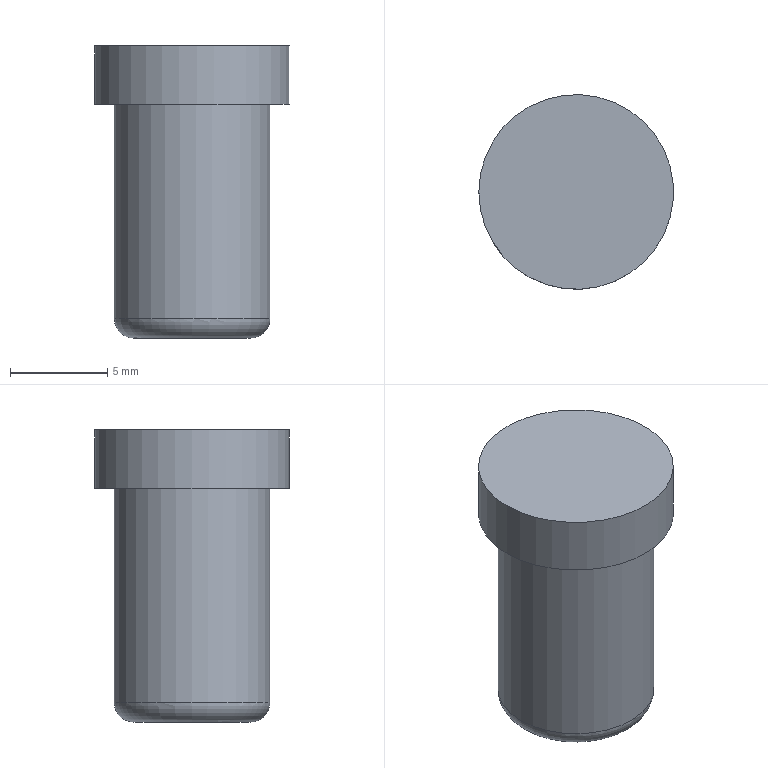Part | STEP file | gslz 2016.10.28-10_id1782_x_t | 1 solid | 6 faces | box 10 x 10 x 15 mm | volume 833.713 mm3 | plane 3 | cylinder 2 | torus 1 | commonest cylinder face diameters 8 x1 10 x1
STEP:
#1=CARTESIAN_POINT('',(0.,0.,0.));
#2=DIRECTION('',(0.,0.,1.));
#3=DIRECTION('',(1.,0.,0.));
#4=AXIS2_PLACEMENT_3D('',#1,#2,#3);
#5=CARTESIAN_POINT('',(815.5,119.5,-4.));
#6=VERTEX_POINT('',#5);
#7=CARTESIAN_POINT('',(819.5,119.5,-4.));
#8=DIRECTION('',(0.,0.,1.));
#9=DIRECTION('',(-1.,0.,0.));
#10=AXIS2_PLACEMENT_3D('',#7,#8,#9);
#11=CIRCLE('',#10,4.);
#12=CARTESIAN_POINT('',(819.5,119.5,-12.));
#13=DIRECTION('',(0.,0.,1.));
#14=DIRECTION('',(1.,0.,0.));
#15=AXIS2_PLACEMENT_3D('',#12,#13,#14);
#16=CYLINDRICAL_SURFACE('',#15,4.);
#17=CARTESIAN_POINT('',(3.142,8.));
#18=DIRECTION('',(1.,0.));
#19=VECTOR('',#18,1.);
#20=LINE('',#17,#19);
#21=(GEOMETRIC_REPRESENTATION_CONTEXT(2)PARAMETRIC_REPRESENTATION_CONTEXT()REPRESENTATION_CONTEXT('',''));
#22=DEFINITIONAL_REPRESENTATION('',(#20),#21);
#23=PCURVE('',#16,#22);
#24=CARTESIAN_POINT('',(819.5,119.5,-4.));
#25=DIRECTION('',(0.,0.,1.));
#26=DIRECTION('',(-1.,0.,0.));
#27=AXIS2_PLACEMENT_3D('',#24,#25,#26);
#28=TOROIDAL_SURFACE('',#27,3.,1.);
#29=CARTESIAN_POINT('',(0.,6.283));
#30=DIRECTION('',(1.,0.));
#31=VECTOR('',#30,1.);
#32=LINE('',#29,#31);
#33=(GEOMETRIC_REPRESENTATION_CONTEXT(2)PARAMETRIC_REPRESENTATION_CONTEXT()REPRESENTATION_CONTEXT('',''));
#34=DEFINITIONAL_REPRESENTATION('',(#32),#33);
#35=PCURVE('',#28,#34);
#36=SURFACE_CURVE('',#11,(#23,#35),.PCURVE_S1.);
#37=EDGE_CURVE('',#6,#6,#36,.T.);
#38=ORIENTED_EDGE('',*,*,#37,.T.);
#39=CARTESIAN_POINT('',(815.5,119.5,7.));
#40=VERTEX_POINT('',#39);
#41=CARTESIAN_POINT('',(815.5,119.5,-4.));
#42=CARTESIAN_POINT('',(815.5,119.5,7.));
#43=B_SPLINE_CURVE_WITH_KNOTS('',1,(#41,#42),.UNSPECIFIED.,.F.,.F.,(2,2),(8.,19.),.PIECEWISE_BEZIER_KNOTS.);
#44=CARTESIAN_POINT('',(9.425,0.));
#45=DIRECTION('',(0.,1.));
#46=VECTOR('',#45,1.);
#47=LINE('',#44,#46);
#48=(GEOMETRIC_REPRESENTATION_CONTEXT(2)PARAMETRIC_REPRESENTATION_CONTEXT()REPRESENTATION_CONTEXT('',''));
#49=DEFINITIONAL_REPRESENTATION('',(#47),#48);
#50=PCURVE('',#16,#49);
#51=CARTESIAN_POINT('',(3.142,0.));
#52=DIRECTION('',(0.,1.));
#53=VECTOR('',#52,1.);
#54=LINE('',#51,#53);
#55=(GEOMETRIC_REPRESENTATION_CONTEXT(2)PARAMETRIC_REPRESENTATION_CONTEXT()REPRESENTATION_CONTEXT('',''));
#56=DEFINITIONAL_REPRESENTATION('',(#54),#55);
#57=PCURVE('',#16,#56);
#58=SEAM_CURVE('',#43,(#50,#57),.PCURVE_S1.);
#59=EDGE_CURVE('',#6,#40,#58,.T.);
#60=ORIENTED_EDGE('',*,*,#59,.T.);
#61=CARTESIAN_POINT('',(819.5,119.5,7.));
#62=DIRECTION('',(0.,0.,1.));
#63=DIRECTION('',(-1.,0.,0.));
#64=AXIS2_PLACEMENT_3D('',#61,#62,#63);
#65=CIRCLE('',#64,4.);
#66=CARTESIAN_POINT('',(3.142,19.));
#67=DIRECTION('',(1.,0.));
#68=VECTOR('',#67,1.);
#69=LINE('',#66,#68);
#70=(GEOMETRIC_REPRESENTATION_CONTEXT(2)PARAMETRIC_REPRESENTATION_CONTEXT()REPRESENTATION_CONTEXT('',''));
#71=DEFINITIONAL_REPRESENTATION('',(#69),#70);
#72=PCURVE('',#16,#71);
#73=CARTESIAN_POINT('',(819.5,119.5,7.));
#74=DIRECTION('',(0.,0.,1.));
#75=DIRECTION('',(1.,0.,0.));
#76=AXIS2_PLACEMENT_3D('',#73,#74,#75);
#77=PLANE('',#76);
#78=CARTESIAN_POINT('',(0.,0.));
#79=DIRECTION('',(-1.,0.));
#80=AXIS2_PLACEMENT_2D('',#78,#79);
#81=CIRCLE('',#80,4.);
#82=(GEOMETRIC_REPRESENTATION_CONTEXT(2)PARAMETRIC_REPRESENTATION_CONTEXT()REPRESENTATION_CONTEXT('',''));
#83=DEFINITIONAL_REPRESENTATION('',(#81),#82);
#84=PCURVE('',#77,#83);
#85=SURFACE_CURVE('',#65,(#72,#84),.PCURVE_S1.);
#86=EDGE_CURVE('',#40,#40,#85,.T.);
#87=ORIENTED_EDGE('',*,*,#86,.F.);
#88=ORIENTED_EDGE('',*,*,#59,.F.);
#89=EDGE_LOOP('',(#38,#60,#87,#88));
#90=FACE_BOUND('',#89,.T.);
#91=ADVANCED_FACE('',(#90),#16,.T.);
#92=CARTESIAN_POINT('',(822.5,119.5,-5.));
#93=VERTEX_POINT('',#92);
#94=CARTESIAN_POINT('',(816.5,119.5,-5.));
#95=VERTEX_POINT('',#94);
#96=CARTESIAN_POINT('',(819.5,119.5,-5.));
#97=DIRECTION('',(0.,0.,-1.));
#98=DIRECTION('',(-1.,0.,0.));
#99=AXIS2_PLACEMENT_3D('',#96,#97,#98);
#100=CIRCLE('',#99,3.);
#101=CARTESIAN_POINT('',(819.5,119.5,-5.));
#102=DIRECTION('',(0.,0.,1.));
#103=DIRECTION('',(1.,0.,0.));
#104=AXIS2_PLACEMENT_3D('',#101,#102,#103);
#105=PLANE('',#104);
#106=CARTESIAN_POINT('',(-3.,0.));
#107=CARTESIAN_POINT('',(-3.,5.196));
#108=CARTESIAN_POINT('',(1.5,2.598));
#109=CARTESIAN_POINT('',(6.,0.));
#110=CARTESIAN_POINT('',(1.5,-2.598));
#111=CARTESIAN_POINT('',(-3.,-5.196));
#112=CARTESIAN_POINT('',(-3.,0.));
#113=(BOUNDED_CURVE()B_SPLINE_CURVE(2,(#106,#107,#108,#109,#110,#111,#112),.UNSPECIFIED.,.T.,.F.)B_SPLINE_CURVE_WITH_KNOTS((1,2,2,2,2,1),(-2.094,0.,2.094,4.189,6.283,8.378),.UNSPECIFIED.)CURVE()GEOMETRIC_REPRESENTATION_ITEM()RATIONAL_B_SPLINE_CURVE((1.,0.5,1.,0.5,1.,0.5,1.))REPRESENTATION_ITEM(''));
#114=(GEOMETRIC_REPRESENTATION_CONTEXT(2)PARAMETRIC_REPRESENTATION_CONTEXT()REPRESENTATION_CONTEXT('',''));
#115=DEFINITIONAL_REPRESENTATION('',(#113),#114);
#116=PCURVE('',#105,#115);
#117=CARTESIAN_POINT('',(6.283,4.712));
#118=DIRECTION('',(-1.,0.));
#119=VECTOR('',#118,1.);
#120=LINE('',#117,#119);
#121=(GEOMETRIC_REPRESENTATION_CONTEXT(2)PARAMETRIC_REPRESENTATION_CONTEXT()REPRESENTATION_CONTEXT('',''));
#122=DEFINITIONAL_REPRESENTATION('',(#120),#121);
#123=PCURVE('',#28,#122);
#124=SURFACE_CURVE('',#100,(#116,#123),.PCURVE_S1.);
#125=EDGE_CURVE('',#93,#95,#124,.T.);
#126=ORIENTED_EDGE('',*,*,#125,.T.);
#127=CARTESIAN_POINT('',(819.5,119.5,-5.));
#128=DIRECTION('',(0.,0.,-1.));
#129=DIRECTION('',(-1.,0.,0.));
#130=AXIS2_PLACEMENT_3D('',#127,#128,#129);
#131=CIRCLE('',#130,3.);
#132=CARTESIAN_POINT('',(-3.,0.));
#133=CARTESIAN_POINT('',(-3.,5.196));
#134=CARTESIAN_POINT('',(1.5,2.598));
#135=CARTESIAN_POINT('',(6.,0.));
#136=CARTESIAN_POINT('',(1.5,-2.598));
#137=CARTESIAN_POINT('',(-3.,-5.196));
#138=CARTESIAN_POINT('',(-3.,0.));
#139=(BOUNDED_CURVE()B_SPLINE_CURVE(2,(#132,#133,#134,#135,#136,#137,#138),.UNSPECIFIED.,.T.,.F.)B_SPLINE_CURVE_WITH_KNOTS((1,2,2,2,2,1),(-2.094,0.,2.094,4.189,6.283,8.378),.UNSPECIFIED.)CURVE()GEOMETRIC_REPRESENTATION_ITEM()RATIONAL_B_SPLINE_CURVE((1.,0.5,1.,0.5,1.,0.5,1.))REPRESENTATION_ITEM(''));
#140=(GEOMETRIC_REPRESENTATION_CONTEXT(2)PARAMETRIC_REPRESENTATION_CONTEXT()REPRESENTATION_CONTEXT('',''));
#141=DEFINITIONAL_REPRESENTATION('',(#139),#140);
#142=PCURVE('',#105,#141);
#143=CARTESIAN_POINT('',(12.566,4.712));
#144=DIRECTION('',(-1.,0.));
#145=VECTOR('',#144,1.);
#146=LINE('',#143,#145);
#147=(GEOMETRIC_REPRESENTATION_CONTEXT(2)PARAMETRIC_REPRESENTATION_CONTEXT()REPRESENTATION_CONTEXT('',''));
#148=DEFINITIONAL_REPRESENTATION('',(#146),#147);
#149=PCURVE('',#28,#148);
#150=SURFACE_CURVE('',#131,(#142,#149),.PCURVE_S1.);
#151=EDGE_CURVE('',#95,#93,#150,.T.);
#152=ORIENTED_EDGE('',*,*,#151,.T.);
#153=EDGE_LOOP('',(#126,#152));
#154=FACE_BOUND('',#153,.T.);
#155=ADVANCED_FACE('',(#154),#105,.F.);
#156=CARTESIAN_POINT('',(814.5,119.5,7.));
#157=VERTEX_POINT('',#156);
#158=CARTESIAN_POINT('',(819.5,119.5,7.));
#159=DIRECTION('',(0.,0.,1.));
#160=DIRECTION('',(-1.,0.,0.));
#161=AXIS2_PLACEMENT_3D('',#158,#159,#160);
#162=CIRCLE('',#161,5.);
#163=CARTESIAN_POINT('',(0.,0.));
#164=DIRECTION('',(-1.,0.));
#165=AXIS2_PLACEMENT_2D('',#163,#164);
#166=CIRCLE('',#165,5.);
#167=(GEOMETRIC_REPRESENTATION_CONTEXT(2)PARAMETRIC_REPRESENTATION_CONTEXT()REPRESENTATION_CONTEXT('',''));
#168=DEFINITIONAL_REPRESENTATION('',(#166),#167);
#169=PCURVE('',#77,#168);
#170=CARTESIAN_POINT('',(819.5,119.5,10.));
#171=DIRECTION('',(0.,0.,-1.));
#172=DIRECTION('',(-1.,0.,0.));
#173=AXIS2_PLACEMENT_3D('',#170,#171,#172);
#174=CYLINDRICAL_SURFACE('',#173,5.);
#175=CARTESIAN_POINT('',(6.283,3.));
#176=DIRECTION('',(-1.,0.));
#177=VECTOR('',#176,1.);
#178=LINE('',#175,#177);
#179=(GEOMETRIC_REPRESENTATION_CONTEXT(2)PARAMETRIC_REPRESENTATION_CONTEXT()REPRESENTATION_CONTEXT('',''));
#180=DEFINITIONAL_REPRESENTATION('',(#178),#179);
#181=PCURVE('',#174,#180);
#182=SURFACE_CURVE('',#162,(#169,#181),.PCURVE_S1.);
#183=EDGE_CURVE('',#157,#157,#182,.T.);
#184=ORIENTED_EDGE('',*,*,#183,.F.);
#185=EDGE_LOOP('',(#184));
#186=FACE_BOUND('',#185,.T.);
#187=ORIENTED_EDGE('',*,*,#86,.T.);
#188=EDGE_LOOP('',(#187));
#189=FACE_BOUND('',#188,.T.);
#190=ADVANCED_FACE('',(#186,#189),#77,.F.);
#191=CARTESIAN_POINT('',(814.5,119.5,10.));
#192=VERTEX_POINT('',#191);
#193=CARTESIAN_POINT('',(819.5,119.5,10.));
#194=DIRECTION('',(0.,0.,1.));
#195=DIRECTION('',(-1.,0.,0.));
#196=AXIS2_PLACEMENT_3D('',#193,#194,#195);
#197=CIRCLE('',#196,5.);
#198=CARTESIAN_POINT('',(6.283,0.));
#199=DIRECTION('',(-1.,0.));
#200=VECTOR('',#199,1.);
#201=LINE('',#198,#200);
#202=(GEOMETRIC_REPRESENTATION_CONTEXT(2)PARAMETRIC_REPRESENTATION_CONTEXT()REPRESENTATION_CONTEXT('',''));
#203=DEFINITIONAL_REPRESENTATION('',(#201),#202);
#204=PCURVE('',#174,#203);
#205=CARTESIAN_POINT('',(819.5,119.5,10.));
#206=DIRECTION('',(0.,0.,1.));
#207=DIRECTION('',(1.,0.,0.));
#208=AXIS2_PLACEMENT_3D('',#205,#206,#207);
#209=PLANE('',#208);
#210=CARTESIAN_POINT('',(0.,0.));
#211=DIRECTION('',(-1.,0.));
#212=AXIS2_PLACEMENT_2D('',#210,#211);
#213=CIRCLE('',#212,5.);
#214=(GEOMETRIC_REPRESENTATION_CONTEXT(2)PARAMETRIC_REPRESENTATION_CONTEXT()REPRESENTATION_CONTEXT('',''));
#215=DEFINITIONAL_REPRESENTATION('',(#213),#214);
#216=PCURVE('',#209,#215);
#217=SURFACE_CURVE('',#197,(#204,#216),.PCURVE_S1.);
#218=EDGE_CURVE('',#192,#192,#217,.T.);
#219=ORIENTED_EDGE('',*,*,#218,.F.);
#220=CARTESIAN_POINT('',(814.5,119.5,10.));
#221=CARTESIAN_POINT('',(814.5,119.5,7.));
#222=B_SPLINE_CURVE_WITH_KNOTS('',1,(#220,#221),.UNSPECIFIED.,.F.,.F.,(2,2),(0.,3.),.PIECEWISE_BEZIER_KNOTS.);
#223=CARTESIAN_POINT('',(6.283,0.));
#224=DIRECTION('',(0.,1.));
#225=VECTOR('',#224,1.);
#226=LINE('',#223,#225);
#227=(GEOMETRIC_REPRESENTATION_CONTEXT(2)PARAMETRIC_REPRESENTATION_CONTEXT()REPRESENTATION_CONTEXT('',''));
#228=DEFINITIONAL_REPRESENTATION('',(#226),#227);
#229=PCURVE('',#174,#228);
#230=CARTESIAN_POINT('',(0.,0.));
#231=DIRECTION('',(0.,1.));
#232=VECTOR('',#231,1.);
#233=LINE('',#230,#232);
#234=(GEOMETRIC_REPRESENTATION_CONTEXT(2)PARAMETRIC_REPRESENTATION_CONTEXT()REPRESENTATION_CONTEXT('',''));
#235=DEFINITIONAL_REPRESENTATION('',(#233),#234);
#236=PCURVE('',#174,#235);
#237=SEAM_CURVE('',#222,(#229,#236),.PCURVE_S1.);
#238=EDGE_CURVE('',#192,#157,#237,.T.);
#239=ORIENTED_EDGE('',*,*,#238,.T.);
#240=ORIENTED_EDGE('',*,*,#183,.T.);
#241=ORIENTED_EDGE('',*,*,#238,.F.);
#242=EDGE_LOOP('',(#219,#239,#240,#241));
#243=FACE_BOUND('',#242,.T.);
#244=ADVANCED_FACE('',(#243),#174,.T.);
#245=ORIENTED_EDGE('',*,*,#218,.T.);
#246=EDGE_LOOP('',(#245));
#247=FACE_BOUND('',#246,.T.);
#248=ADVANCED_FACE('',(#247),#209,.T.);
#249=ORIENTED_EDGE('',*,*,#151,.F.);
#250=CARTESIAN_POINT('',(816.5,119.5,-5.));
#251=CARTESIAN_POINT('',(816.233,119.5,-5.));
#252=CARTESIAN_POINT('',(815.972,119.5,-4.915));
#253=CARTESIAN_POINT('',(815.748,119.5,-4.752));
#254=CARTESIAN_POINT('',(815.585,119.5,-4.528));
#255=CARTESIAN_POINT('',(815.5,119.5,-4.267));
#256=CARTESIAN_POINT('',(815.5,119.5,-4.));
#257=(BOUNDED_CURVE()B_SPLINE_CURVE(6,(#250,#251,#252,#253,#254,#255,#256),.UNSPECIFIED.,.F.,.F.)B_SPLINE_CURVE_WITH_KNOTS((7,7),(4.712,6.283),.PIECEWISE_BEZIER_KNOTS.)CURVE()GEOMETRIC_REPRESENTATION_ITEM()RATIONAL_B_SPLINE_CURVE((1.031,1.01,0.9979,0.994,0.9979,1.01,1.031))REPRESENTATION_ITEM(''));
#258=CARTESIAN_POINT('',(6.283,0.));
#259=DIRECTION('',(0.,1.));
#260=VECTOR('',#259,1.);
#261=LINE('',#258,#260);
#262=(GEOMETRIC_REPRESENTATION_CONTEXT(2)PARAMETRIC_REPRESENTATION_CONTEXT()REPRESENTATION_CONTEXT('',''));
#263=DEFINITIONAL_REPRESENTATION('',(#261),#262);
#264=PCURVE('',#28,#263);
#265=CARTESIAN_POINT('',(0.,0.));
#266=DIRECTION('',(0.,1.));
#267=VECTOR('',#266,1.);
#268=LINE('',#265,#267);
#269=(GEOMETRIC_REPRESENTATION_CONTEXT(2)PARAMETRIC_REPRESENTATION_CONTEXT()REPRESENTATION_CONTEXT('',''));
#270=DEFINITIONAL_REPRESENTATION('',(#268),#269);
#271=PCURVE('',#28,#270);
#272=SEAM_CURVE('',#257,(#264,#271),.PCURVE_S1.);
#273=EDGE_CURVE('',#95,#6,#272,.T.);
#274=ORIENTED_EDGE('',*,*,#273,.T.);
#275=ORIENTED_EDGE('',*,*,#37,.F.);
#276=ORIENTED_EDGE('',*,*,#273,.F.);
#277=ORIENTED_EDGE('',*,*,#125,.F.);
#278=EDGE_LOOP('',(#249,#274,#275,#276,#277));
#279=FACE_BOUND('',#278,.T.);
#280=ADVANCED_FACE('',(#279),#28,.T.);
#281=CLOSED_SHELL('',(#91,#155,#190,#244,#248,#280));
#282=MANIFOLD_SOLID_BREP('',#281);
#283=(LENGTH_UNIT()NAMED_UNIT(*)SI_UNIT(.MILLI.,.METRE.));
#284=UNCERTAINTY_MEASURE_WITH_UNIT(LENGTH_MEASURE(0.000005),#283,'','');
#285=(NAMED_UNIT(*)PLANE_ANGLE_UNIT()SI_UNIT($,.RADIAN.));
#286=(NAMED_UNIT(*)SI_UNIT($,.STERADIAN.)SOLID_ANGLE_UNIT());
#287=(GEOMETRIC_REPRESENTATION_CONTEXT(3)GLOBAL_UNCERTAINTY_ASSIGNED_CONTEXT((#284))GLOBAL_UNIT_ASSIGNED_CONTEXT((#283,#285,#286))REPRESENTATION_CONTEXT('',''));
#288=ADVANCED_BREP_SHAPE_REPRESENTATION('',(#4,#282),#287);